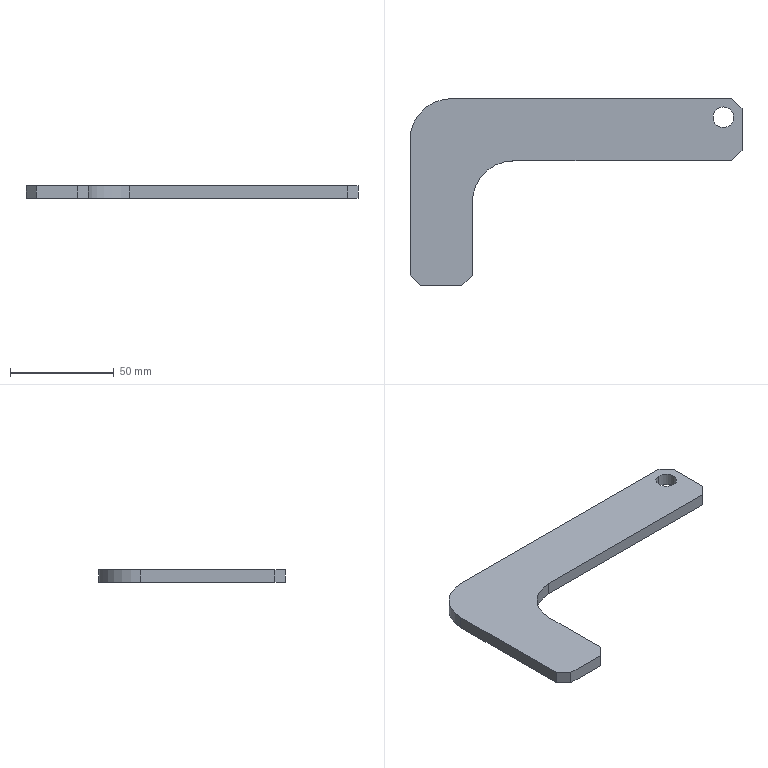Part | STEP file | [02]-8 | 1 solid | 16 faces | box 160 x 90 x 6 mm | volume 38829 mm3 | plane 12 | cylinder 4 | commonest cylinder face diameters 10 x2 40 x2
STEP:
#1=CARTESIAN_POINT('',(151.,-4.,6.));
#2=VERTEX_POINT('',#1);
#3=CARTESIAN_POINT('',(151.,-14.,6.));
#4=VERTEX_POINT('',#3);
#5=CARTESIAN_POINT('',(151.,-9.,6.));
#6=DIRECTION('',(0.,0.,-1.));
#7=DIRECTION('',(0.,-1.,0.));
#8=AXIS2_PLACEMENT_3D('',#5,#6,#7);
#9=CIRCLE('',#8,5.);
#10=EDGE_CURVE('',#2,#4,#9,.T.);
#11=ORIENTED_EDGE('',*,*,#10,.F.);
#12=CARTESIAN_POINT('',(151.,-4.,0.));
#13=VERTEX_POINT('',#12);
#14=CARTESIAN_POINT('',(151.,-4.,6.));
#15=DIRECTION('',(0.,0.,-1.));
#16=VECTOR('',#15,1000.);
#17=LINE('',#14,#16);
#18=EDGE_CURVE('',#2,#13,#17,.T.);
#19=ORIENTED_EDGE('',*,*,#18,.T.);
#20=CARTESIAN_POINT('',(151.,-14.,0.));
#21=VERTEX_POINT('',#20);
#22=CARTESIAN_POINT('',(151.,-9.,0.));
#23=DIRECTION('',(0.,0.,1.));
#24=DIRECTION('',(0.,1.,0.));
#25=AXIS2_PLACEMENT_3D('',#22,#23,#24);
#26=CIRCLE('',#25,5.);
#27=EDGE_CURVE('',#21,#13,#26,.T.);
#28=ORIENTED_EDGE('',*,*,#27,.F.);
#29=CARTESIAN_POINT('',(151.,-14.,6.));
#30=DIRECTION('',(0.,0.,-1.));
#31=VECTOR('',#30,1000.);
#32=LINE('',#29,#31);
#33=EDGE_CURVE('',#4,#21,#32,.T.);
#34=ORIENTED_EDGE('',*,*,#33,.F.);
#35=EDGE_LOOP('',(#11,#19,#28,#34));
#36=FACE_OUTER_BOUND('',#35,.T.);
#37=CARTESIAN_POINT('',(151.,-9.,6.));
#38=DIRECTION('',(0.,0.,-1.));
#39=DIRECTION('',(0.,-1.,0.));
#40=AXIS2_PLACEMENT_3D('',#37,#38,#39);
#41=CYLINDRICAL_SURFACE('',#40,5.);
#42=ADVANCED_FACE('',(#36),#41,.F.);
#43=CARTESIAN_POINT('',(50.,-30.,6.));
#44=VERTEX_POINT('',#43);
#45=CARTESIAN_POINT('',(155.,-30.,6.));
#46=VERTEX_POINT('',#45);
#47=CARTESIAN_POINT('',(80.,-30.,6.));
#48=DIRECTION('',(1.,0.,0.));
#49=VECTOR('',#48,1000.);
#50=LINE('',#47,#49);
#51=EDGE_CURVE('',#44,#46,#50,.T.);
#52=ORIENTED_EDGE('',*,*,#51,.F.);
#53=CARTESIAN_POINT('',(50.,-30.,0.));
#54=VERTEX_POINT('',#53);
#55=CARTESIAN_POINT('',(50.,-30.,6.));
#56=DIRECTION('',(0.,0.,1.));
#57=VECTOR('',#56,1000.);
#58=LINE('',#55,#57);
#59=EDGE_CURVE('',#54,#44,#58,.T.);
#60=ORIENTED_EDGE('',*,*,#59,.F.);
#61=CARTESIAN_POINT('',(155.,-30.,0.));
#62=VERTEX_POINT('',#61);
#63=CARTESIAN_POINT('',(80.,-30.,0.));
#64=DIRECTION('',(-1.,0.,0.));
#65=VECTOR('',#64,1000.);
#66=LINE('',#63,#65);
#67=EDGE_CURVE('',#62,#54,#66,.T.);
#68=ORIENTED_EDGE('',*,*,#67,.F.);
#69=CARTESIAN_POINT('',(155.,-30.,0.));
#70=DIRECTION('',(0.,0.,-1.));
#71=VECTOR('',#70,1000.);
#72=LINE('',#69,#71);
#73=EDGE_CURVE('',#46,#62,#72,.T.);
#74=ORIENTED_EDGE('',*,*,#73,.F.);
#75=EDGE_LOOP('',(#52,#60,#68,#74));
#76=FACE_OUTER_BOUND('',#75,.T.);
#77=CARTESIAN_POINT('',(80.,-30.,0.));
#78=DIRECTION('',(0.,-1.,0.));
#79=DIRECTION('',(0.,0.,1.));
#80=AXIS2_PLACEMENT_3D('',#77,#78,#79);
#81=PLANE('',#80);
#82=ADVANCED_FACE('',(#76),#81,.T.);
#83=CARTESIAN_POINT('',(151.,-9.,6.));
#84=DIRECTION('',(0.,0.,-1.));
#85=DIRECTION('',(0.,-1.,0.));
#86=AXIS2_PLACEMENT_3D('',#83,#84,#85);
#87=CIRCLE('',#86,5.);
#88=EDGE_CURVE('',#4,#2,#87,.T.);
#89=ORIENTED_EDGE('',*,*,#88,.T.);
#90=ORIENTED_EDGE('',*,*,#10,.T.);
#91=EDGE_LOOP('',(#89,#90));
#92=FACE_BOUND('',#91,.T.);
#93=CARTESIAN_POINT('',(0.,-20.,6.));
#94=VERTEX_POINT('',#93);
#95=CARTESIAN_POINT('',(0.,-85.,6.));
#96=VERTEX_POINT('',#95);
#97=CARTESIAN_POINT('',(0.,-15.,6.));
#98=DIRECTION('',(0.,-1.,0.));
#99=VECTOR('',#98,1000.);
#100=LINE('',#97,#99);
#101=EDGE_CURVE('',#94,#96,#100,.T.);
#102=ORIENTED_EDGE('',*,*,#101,.T.);
#103=CARTESIAN_POINT('',(5.,-90.,6.));
#104=VERTEX_POINT('',#103);
#105=CARTESIAN_POINT('',(5.,-90.,6.));
#106=DIRECTION('',(-0.7071,0.7071,0.));
#107=VECTOR('',#106,1000.);
#108=LINE('',#105,#107);
#109=EDGE_CURVE('',#104,#96,#108,.T.);
#110=ORIENTED_EDGE('',*,*,#109,.F.);
#111=CARTESIAN_POINT('',(25.,-90.,6.));
#112=VERTEX_POINT('',#111);
#113=CARTESIAN_POINT('',(15.,-90.,6.));
#114=DIRECTION('',(1.,0.,0.));
#115=VECTOR('',#114,1000.);
#116=LINE('',#113,#115);
#117=EDGE_CURVE('',#104,#112,#116,.T.);
#118=ORIENTED_EDGE('',*,*,#117,.T.);
#119=CARTESIAN_POINT('',(30.,-85.,6.));
#120=VERTEX_POINT('',#119);
#121=CARTESIAN_POINT('',(90.,-25.,6.));
#122=DIRECTION('',(-0.7071,-0.7071,0.));
#123=VECTOR('',#122,1000.);
#124=LINE('',#121,#123);
#125=EDGE_CURVE('',#120,#112,#124,.T.);
#126=ORIENTED_EDGE('',*,*,#125,.F.);
#127=CARTESIAN_POINT('',(30.,-50.,6.));
#128=VERTEX_POINT('',#127);
#129=CARTESIAN_POINT('',(30.,-60.,6.));
#130=DIRECTION('',(0.,1.,0.));
#131=VECTOR('',#130,1000.);
#132=LINE('',#129,#131);
#133=EDGE_CURVE('',#120,#128,#132,.T.);
#134=ORIENTED_EDGE('',*,*,#133,.T.);
#135=CARTESIAN_POINT('',(50.,-50.,6.));
#136=DIRECTION('',(0.,0.,1.));
#137=DIRECTION('',(0.,1.,0.));
#138=AXIS2_PLACEMENT_3D('',#135,#136,#137);
#139=CIRCLE('',#138,20.);
#140=EDGE_CURVE('',#44,#128,#139,.T.);
#141=ORIENTED_EDGE('',*,*,#140,.F.);
#142=ORIENTED_EDGE('',*,*,#51,.T.);
#143=CARTESIAN_POINT('',(160.,-25.,6.));
#144=VERTEX_POINT('',#143);
#145=CARTESIAN_POINT('',(125.,-60.,6.));
#146=DIRECTION('',(-0.7071,-0.7071,0.));
#147=VECTOR('',#146,1000.);
#148=LINE('',#145,#147);
#149=EDGE_CURVE('',#144,#46,#148,.T.);
#150=ORIENTED_EDGE('',*,*,#149,.F.);
#151=CARTESIAN_POINT('',(160.,-5.,6.));
#152=VERTEX_POINT('',#151);
#153=CARTESIAN_POINT('',(160.,-15.,6.));
#154=DIRECTION('',(0.,1.,0.));
#155=VECTOR('',#154,1000.);
#156=LINE('',#153,#155);
#157=EDGE_CURVE('',#144,#152,#156,.T.);
#158=ORIENTED_EDGE('',*,*,#157,.T.);
#159=CARTESIAN_POINT('',(155.,0.,6.));
#160=VERTEX_POINT('',#159);
#161=CARTESIAN_POINT('',(125.,30.,6.));
#162=DIRECTION('',(0.7071,-0.7071,0.));
#163=VECTOR('',#162,1000.);
#164=LINE('',#161,#163);
#165=EDGE_CURVE('',#160,#152,#164,.T.);
#166=ORIENTED_EDGE('',*,*,#165,.F.);
#167=CARTESIAN_POINT('',(20.,0.,6.));
#168=VERTEX_POINT('',#167);
#169=CARTESIAN_POINT('',(80.,0.,6.));
#170=DIRECTION('',(-1.,0.,0.));
#171=VECTOR('',#170,1000.);
#172=LINE('',#169,#171);
#173=EDGE_CURVE('',#160,#168,#172,.T.);
#174=ORIENTED_EDGE('',*,*,#173,.T.);
#175=CARTESIAN_POINT('',(20.,-20.,6.));
#176=DIRECTION('',(0.,0.,-1.));
#177=DIRECTION('',(0.,1.,0.));
#178=AXIS2_PLACEMENT_3D('',#175,#176,#177);
#179=CIRCLE('',#178,20.);
#180=EDGE_CURVE('',#94,#168,#179,.T.);
#181=ORIENTED_EDGE('',*,*,#180,.F.);
#182=EDGE_LOOP('',(#102,#110,#118,#126,#134,#141,#142,#150,#158,#166,#174,#181));
#183=FACE_OUTER_BOUND('',#182,.T.);
#184=CARTESIAN_POINT('',(80.,-15.,6.));
#185=DIRECTION('',(0.,0.,1.));
#186=DIRECTION('',(0.,1.,0.));
#187=AXIS2_PLACEMENT_3D('',#184,#185,#186);
#188=PLANE('',#187);
#189=ADVANCED_FACE('',(#92,#183),#188,.T.);
#190=CARTESIAN_POINT('',(0.,-85.,0.));
#191=VERTEX_POINT('',#190);
#192=CARTESIAN_POINT('',(0.,-20.,0.));
#193=VERTEX_POINT('',#192);
#194=CARTESIAN_POINT('',(0.,-15.,0.));
#195=DIRECTION('',(0.,1.,0.));
#196=VECTOR('',#195,1000.);
#197=LINE('',#194,#196);
#198=EDGE_CURVE('',#191,#193,#197,.T.);
#199=ORIENTED_EDGE('',*,*,#198,.F.);
#200=CARTESIAN_POINT('',(0.,-85.,0.));
#201=DIRECTION('',(0.,0.,-1.));
#202=VECTOR('',#201,1000.);
#203=LINE('',#200,#202);
#204=EDGE_CURVE('',#96,#191,#203,.T.);
#205=ORIENTED_EDGE('',*,*,#204,.F.);
#206=ORIENTED_EDGE('',*,*,#101,.F.);
#207=CARTESIAN_POINT('',(0.,-20.,0.));
#208=DIRECTION('',(0.,0.,1.));
#209=VECTOR('',#208,1000.);
#210=LINE('',#207,#209);
#211=EDGE_CURVE('',#193,#94,#210,.T.);
#212=ORIENTED_EDGE('',*,*,#211,.F.);
#213=EDGE_LOOP('',(#199,#205,#206,#212));
#214=FACE_OUTER_BOUND('',#213,.T.);
#215=CARTESIAN_POINT('',(0.,-15.,0.));
#216=DIRECTION('',(-1.,0.,0.));
#217=DIRECTION('',(0.,0.,-1.));
#218=AXIS2_PLACEMENT_3D('',#215,#216,#217);
#219=PLANE('',#218);
#220=ADVANCED_FACE('',(#214),#219,.T.);
#221=CARTESIAN_POINT('',(160.,-5.,0.));
#222=VERTEX_POINT('',#221);
#223=CARTESIAN_POINT('',(160.,-25.,0.));
#224=VERTEX_POINT('',#223);
#225=CARTESIAN_POINT('',(160.,-15.,0.));
#226=DIRECTION('',(0.,-1.,0.));
#227=VECTOR('',#226,1000.);
#228=LINE('',#225,#227);
#229=EDGE_CURVE('',#222,#224,#228,.T.);
#230=ORIENTED_EDGE('',*,*,#229,.F.);
#231=CARTESIAN_POINT('',(160.,-5.,0.));
#232=DIRECTION('',(0.,0.,-1.));
#233=VECTOR('',#232,1000.);
#234=LINE('',#231,#233);
#235=EDGE_CURVE('',#152,#222,#234,.T.);
#236=ORIENTED_EDGE('',*,*,#235,.F.);
#237=ORIENTED_EDGE('',*,*,#157,.F.);
#238=CARTESIAN_POINT('',(160.,-25.,0.));
#239=DIRECTION('',(0.,0.,1.));
#240=VECTOR('',#239,1000.);
#241=LINE('',#238,#240);
#242=EDGE_CURVE('',#224,#144,#241,.T.);
#243=ORIENTED_EDGE('',*,*,#242,.F.);
#244=EDGE_LOOP('',(#230,#236,#237,#243));
#245=FACE_OUTER_BOUND('',#244,.T.);
#246=CARTESIAN_POINT('',(160.,-15.,0.));
#247=DIRECTION('',(1.,0.,0.));
#248=DIRECTION('',(0.,0.,1.));
#249=AXIS2_PLACEMENT_3D('',#246,#247,#248);
#250=PLANE('',#249);
#251=ADVANCED_FACE('',(#245),#250,.T.);
#252=ORIENTED_EDGE('',*,*,#27,.T.);
#253=CARTESIAN_POINT('',(151.,-9.,0.));
#254=DIRECTION('',(0.,0.,1.));
#255=DIRECTION('',(0.,1.,0.));
#256=AXIS2_PLACEMENT_3D('',#253,#254,#255);
#257=CIRCLE('',#256,5.);
#258=EDGE_CURVE('',#13,#21,#257,.T.);
#259=ORIENTED_EDGE('',*,*,#258,.T.);
#260=EDGE_LOOP('',(#252,#259));
#261=FACE_BOUND('',#260,.T.);
#262=CARTESIAN_POINT('',(20.,0.,0.));
#263=VERTEX_POINT('',#262);
#264=CARTESIAN_POINT('',(155.,0.,0.));
#265=VERTEX_POINT('',#264);
#266=CARTESIAN_POINT('',(80.,0.,0.));
#267=DIRECTION('',(1.,0.,0.));
#268=VECTOR('',#267,1000.);
#269=LINE('',#266,#268);
#270=EDGE_CURVE('',#263,#265,#269,.T.);
#271=ORIENTED_EDGE('',*,*,#270,.T.);
#272=CARTESIAN_POINT('',(125.,30.,0.));
#273=DIRECTION('',(-0.7071,0.7071,0.));
#274=VECTOR('',#273,1000.);
#275=LINE('',#272,#274);
#276=EDGE_CURVE('',#222,#265,#275,.T.);
#277=ORIENTED_EDGE('',*,*,#276,.F.);
#278=ORIENTED_EDGE('',*,*,#229,.T.);
#279=CARTESIAN_POINT('',(125.,-60.,0.));
#280=DIRECTION('',(0.7071,0.7071,0.));
#281=VECTOR('',#280,1000.);
#282=LINE('',#279,#281);
#283=EDGE_CURVE('',#62,#224,#282,.T.);
#284=ORIENTED_EDGE('',*,*,#283,.F.);
#285=ORIENTED_EDGE('',*,*,#67,.T.);
#286=CARTESIAN_POINT('',(30.,-50.,0.));
#287=VERTEX_POINT('',#286);
#288=CARTESIAN_POINT('',(50.,-50.,0.));
#289=DIRECTION('',(0.,0.,-1.));
#290=DIRECTION('',(0.,-1.,0.));
#291=AXIS2_PLACEMENT_3D('',#288,#289,#290);
#292=CIRCLE('',#291,20.);
#293=EDGE_CURVE('',#287,#54,#292,.T.);
#294=ORIENTED_EDGE('',*,*,#293,.F.);
#295=CARTESIAN_POINT('',(30.,-85.,0.));
#296=VERTEX_POINT('',#295);
#297=CARTESIAN_POINT('',(30.,-60.,0.));
#298=DIRECTION('',(0.,-1.,0.));
#299=VECTOR('',#298,1000.);
#300=LINE('',#297,#299);
#301=EDGE_CURVE('',#287,#296,#300,.T.);
#302=ORIENTED_EDGE('',*,*,#301,.T.);
#303=CARTESIAN_POINT('',(25.,-90.,0.));
#304=VERTEX_POINT('',#303);
#305=CARTESIAN_POINT('',(90.,-25.,0.));
#306=DIRECTION('',(0.7071,0.7071,0.));
#307=VECTOR('',#306,1000.);
#308=LINE('',#305,#307);
#309=EDGE_CURVE('',#304,#296,#308,.T.);
#310=ORIENTED_EDGE('',*,*,#309,.F.);
#311=CARTESIAN_POINT('',(5.,-90.,0.));
#312=VERTEX_POINT('',#311);
#313=CARTESIAN_POINT('',(15.,-90.,0.));
#314=DIRECTION('',(-1.,0.,0.));
#315=VECTOR('',#314,1000.);
#316=LINE('',#313,#315);
#317=EDGE_CURVE('',#304,#312,#316,.T.);
#318=ORIENTED_EDGE('',*,*,#317,.T.);
#319=CARTESIAN_POINT('',(5.,-90.,0.));
#320=DIRECTION('',(0.7071,-0.7071,0.));
#321=VECTOR('',#320,1000.);
#322=LINE('',#319,#321);
#323=EDGE_CURVE('',#191,#312,#322,.T.);
#324=ORIENTED_EDGE('',*,*,#323,.F.);
#325=ORIENTED_EDGE('',*,*,#198,.T.);
#326=CARTESIAN_POINT('',(20.,-20.,0.));
#327=DIRECTION('',(0.,0.,1.));
#328=DIRECTION('',(0.,-1.,0.));
#329=AXIS2_PLACEMENT_3D('',#326,#327,#328);
#330=CIRCLE('',#329,20.);
#331=EDGE_CURVE('',#263,#193,#330,.T.);
#332=ORIENTED_EDGE('',*,*,#331,.F.);
#333=EDGE_LOOP('',(#271,#277,#278,#284,#285,#294,#302,#310,#318,#324,#325,#332));
#334=FACE_OUTER_BOUND('',#333,.T.);
#335=CARTESIAN_POINT('',(80.,-15.,0.));
#336=DIRECTION('',(0.,0.,-1.));
#337=DIRECTION('',(0.,-1.,0.));
#338=AXIS2_PLACEMENT_3D('',#335,#336,#337);
#339=PLANE('',#338);
#340=ADVANCED_FACE('',(#261,#334),#339,.T.);
#341=ORIENTED_EDGE('',*,*,#173,.F.);
#342=CARTESIAN_POINT('',(155.,0.,0.));
#343=DIRECTION('',(0.,0.,1.));
#344=VECTOR('',#343,1000.);
#345=LINE('',#342,#344);
#346=EDGE_CURVE('',#265,#160,#345,.T.);
#347=ORIENTED_EDGE('',*,*,#346,.F.);
#348=ORIENTED_EDGE('',*,*,#270,.F.);
#349=CARTESIAN_POINT('',(20.,0.,0.));
#350=DIRECTION('',(0.,0.,-1.));
#351=VECTOR('',#350,1000.);
#352=LINE('',#349,#351);
#353=EDGE_CURVE('',#168,#263,#352,.T.);
#354=ORIENTED_EDGE('',*,*,#353,.F.);
#355=EDGE_LOOP('',(#341,#347,#348,#354));
#356=FACE_OUTER_BOUND('',#355,.T.);
#357=CARTESIAN_POINT('',(80.,0.,0.));
#358=DIRECTION('',(0.,1.,0.));
#359=DIRECTION('',(0.,0.,-1.));
#360=AXIS2_PLACEMENT_3D('',#357,#358,#359);
#361=PLANE('',#360);
#362=ADVANCED_FACE('',(#356),#361,.T.);
#363=ORIENTED_EDGE('',*,*,#317,.F.);
#364=CARTESIAN_POINT('',(25.,-90.,0.));
#365=DIRECTION('',(0.,0.,-1.));
#366=VECTOR('',#365,1000.);
#367=LINE('',#364,#366);
#368=EDGE_CURVE('',#112,#304,#367,.T.);
#369=ORIENTED_EDGE('',*,*,#368,.F.);
#370=ORIENTED_EDGE('',*,*,#117,.F.);
#371=CARTESIAN_POINT('',(5.,-90.,0.));
#372=DIRECTION('',(0.,0.,1.));
#373=VECTOR('',#372,1000.);
#374=LINE('',#371,#373);
#375=EDGE_CURVE('',#312,#104,#374,.T.);
#376=ORIENTED_EDGE('',*,*,#375,.F.);
#377=EDGE_LOOP('',(#363,#369,#370,#376));
#378=FACE_OUTER_BOUND('',#377,.T.);
#379=CARTESIAN_POINT('',(15.,-90.,0.));
#380=DIRECTION('',(0.,-1.,0.));
#381=DIRECTION('',(0.,0.,1.));
#382=AXIS2_PLACEMENT_3D('',#379,#380,#381);
#383=PLANE('',#382);
#384=ADVANCED_FACE('',(#378),#383,.T.);
#385=ORIENTED_EDGE('',*,*,#301,.F.);
#386=CARTESIAN_POINT('',(30.,-50.,0.));
#387=DIRECTION('',(0.,0.,-1.));
#388=VECTOR('',#387,1000.);
#389=LINE('',#386,#388);
#390=EDGE_CURVE('',#128,#287,#389,.T.);
#391=ORIENTED_EDGE('',*,*,#390,.F.);
#392=ORIENTED_EDGE('',*,*,#133,.F.);
#393=CARTESIAN_POINT('',(30.,-85.,0.));
#394=DIRECTION('',(0.,0.,1.));
#395=VECTOR('',#394,1000.);
#396=LINE('',#393,#395);
#397=EDGE_CURVE('',#296,#120,#396,.T.);
#398=ORIENTED_EDGE('',*,*,#397,.F.);
#399=EDGE_LOOP('',(#385,#391,#392,#398));
#400=FACE_OUTER_BOUND('',#399,.T.);
#401=CARTESIAN_POINT('',(30.,-60.,0.));
#402=DIRECTION('',(1.,0.,0.));
#403=DIRECTION('',(0.,0.,1.));
#404=AXIS2_PLACEMENT_3D('',#401,#402,#403);
#405=PLANE('',#404);
#406=ADVANCED_FACE('',(#400),#405,.T.);
#407=ORIENTED_EDGE('',*,*,#293,.T.);
#408=ORIENTED_EDGE('',*,*,#59,.T.);
#409=ORIENTED_EDGE('',*,*,#140,.T.);
#410=ORIENTED_EDGE('',*,*,#390,.T.);
#411=EDGE_LOOP('',(#407,#408,#409,#410));
#412=FACE_OUTER_BOUND('',#411,.T.);
#413=CARTESIAN_POINT('',(50.,-50.,0.));
#414=DIRECTION('',(0.,0.,-1.));
#415=DIRECTION('',(0.,-1.,0.));
#416=AXIS2_PLACEMENT_3D('',#413,#414,#415);
#417=CYLINDRICAL_SURFACE('',#416,20.);
#418=ADVANCED_FACE('',(#412),#417,.F.);
#419=ORIENTED_EDGE('',*,*,#309,.T.);
#420=ORIENTED_EDGE('',*,*,#397,.T.);
#421=ORIENTED_EDGE('',*,*,#125,.T.);
#422=ORIENTED_EDGE('',*,*,#368,.T.);
#423=EDGE_LOOP('',(#419,#420,#421,#422));
#424=FACE_OUTER_BOUND('',#423,.T.);
#425=CARTESIAN_POINT('',(30.,-85.,0.));
#426=DIRECTION('',(-0.7071,0.7071,0.));
#427=DIRECTION('',(0.,0.,1.));
#428=AXIS2_PLACEMENT_3D('',#425,#426,#427);
#429=PLANE('',#428);
#430=ADVANCED_FACE('',(#424),#429,.F.);
#431=ORIENTED_EDGE('',*,*,#323,.T.);
#432=ORIENTED_EDGE('',*,*,#375,.T.);
#433=ORIENTED_EDGE('',*,*,#109,.T.);
#434=ORIENTED_EDGE('',*,*,#204,.T.);
#435=EDGE_LOOP('',(#431,#432,#433,#434));
#436=FACE_OUTER_BOUND('',#435,.T.);
#437=CARTESIAN_POINT('',(5.,-90.,0.));
#438=DIRECTION('',(0.7071,0.7071,0.));
#439=DIRECTION('',(0.,0.,1.));
#440=AXIS2_PLACEMENT_3D('',#437,#438,#439);
#441=PLANE('',#440);
#442=ADVANCED_FACE('',(#436),#441,.F.);
#443=ORIENTED_EDGE('',*,*,#276,.T.);
#444=ORIENTED_EDGE('',*,*,#346,.T.);
#445=ORIENTED_EDGE('',*,*,#165,.T.);
#446=ORIENTED_EDGE('',*,*,#235,.T.);
#447=EDGE_LOOP('',(#443,#444,#445,#446));
#448=FACE_OUTER_BOUND('',#447,.T.);
#449=CARTESIAN_POINT('',(155.,0.,0.));
#450=DIRECTION('',(-0.7071,-0.7071,0.));
#451=DIRECTION('',(0.,0.,1.));
#452=AXIS2_PLACEMENT_3D('',#449,#450,#451);
#453=PLANE('',#452);
#454=ADVANCED_FACE('',(#448),#453,.F.);
#455=ORIENTED_EDGE('',*,*,#283,.T.);
#456=ORIENTED_EDGE('',*,*,#242,.T.);
#457=ORIENTED_EDGE('',*,*,#149,.T.);
#458=ORIENTED_EDGE('',*,*,#73,.T.);
#459=EDGE_LOOP('',(#455,#456,#457,#458));
#460=FACE_OUTER_BOUND('',#459,.T.);
#461=CARTESIAN_POINT('',(160.,-25.,0.));
#462=DIRECTION('',(-0.7071,0.7071,0.));
#463=DIRECTION('',(0.,0.,1.));
#464=AXIS2_PLACEMENT_3D('',#461,#462,#463);
#465=PLANE('',#464);
#466=ADVANCED_FACE('',(#460),#465,.F.);
#467=ORIENTED_EDGE('',*,*,#331,.T.);
#468=ORIENTED_EDGE('',*,*,#211,.T.);
#469=ORIENTED_EDGE('',*,*,#180,.T.);
#470=ORIENTED_EDGE('',*,*,#353,.T.);
#471=EDGE_LOOP('',(#467,#468,#469,#470));
#472=FACE_OUTER_BOUND('',#471,.T.);
#473=CARTESIAN_POINT('',(20.,-20.,0.));
#474=DIRECTION('',(0.,0.,1.));
#475=DIRECTION('',(0.,1.,0.));
#476=AXIS2_PLACEMENT_3D('',#473,#474,#475);
#477=CYLINDRICAL_SURFACE('',#476,20.);
#478=ADVANCED_FACE('',(#472),#477,.T.);
#479=ORIENTED_EDGE('',*,*,#18,.F.);
#480=ORIENTED_EDGE('',*,*,#88,.F.);
#481=ORIENTED_EDGE('',*,*,#33,.T.);
#482=ORIENTED_EDGE('',*,*,#258,.F.);
#483=EDGE_LOOP('',(#479,#480,#481,#482));
#484=FACE_OUTER_BOUND('',#483,.T.);
#485=CARTESIAN_POINT('',(151.,-9.,6.));
#486=DIRECTION('',(0.,0.,-1.));
#487=DIRECTION('',(0.,-1.,0.));
#488=AXIS2_PLACEMENT_3D('',#485,#486,#487);
#489=CYLINDRICAL_SURFACE('',#488,5.);
#490=ADVANCED_FACE('',(#484),#489,.F.);
#491=CLOSED_SHELL('',(#42,#82,#189,#220,#251,#340,#362,#384,#406,#418,#430,#442,#454,#466,#478,#490));
#492=MANIFOLD_SOLID_BREP('',#491);
#493=CARTESIAN_POINT('',(0.,0.,0.));
#494=DIRECTION('',(0.,0.,1.));
#495=DIRECTION('',(1.,0.,0.));
#496=AXIS2_PLACEMENT_3D('',#493,#494,#495);
#497=(LENGTH_UNIT()NAMED_UNIT(*)SI_UNIT(.MILLI.,.METRE.));
#498=UNCERTAINTY_MEASURE_WITH_UNIT(LENGTH_MEASURE(0.00001),#497,'','');
#499=(NAMED_UNIT(*)PLANE_ANGLE_UNIT()SI_UNIT($,.RADIAN.));
#500=(NAMED_UNIT(*)SI_UNIT($,.STERADIAN.)SOLID_ANGLE_UNIT());
#501=(GEOMETRIC_REPRESENTATION_CONTEXT(3)GLOBAL_UNCERTAINTY_ASSIGNED_CONTEXT((#498))GLOBAL_UNIT_ASSIGNED_CONTEXT((#497,#499,#500))REPRESENTATION_CONTEXT('',''));
#502=ADVANCED_BREP_SHAPE_REPRESENTATION('',(#492,#496),#501);